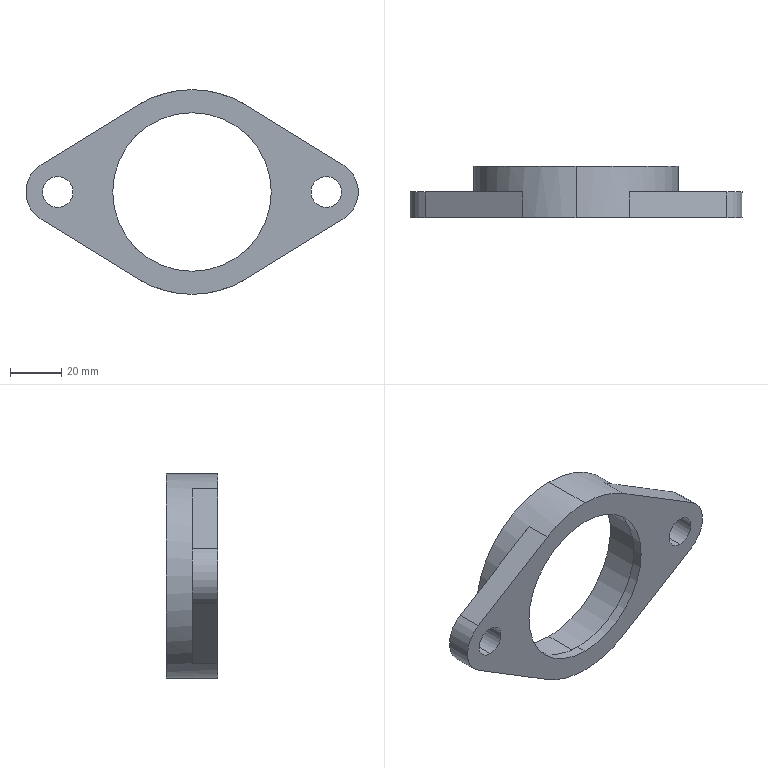Part | SolidWorks | features ICE 3, Extrusion 1 | 1 solid | 21 faces | box 130 x 20 x 80 mm | volume 45606 mm3 | cylinder 12 | plane 9 | commonest cylinder face diameters 12 x4 25 x2 62 x2 68 x2 80 x2
STEP:
#1=CARTESIAN_POINT('',(0.,0.,-31.));
#2=VERTEX_POINT('',#1);
#3=CARTESIAN_POINT('',(0.,0.,31.));
#4=VERTEX_POINT('',#3);
#5=CARTESIAN_POINT('',(0.,0.,0.));
#6=DIRECTION('',(0.,1.,0.));
#7=DIRECTION('',(0.,0.,1.));
#8=AXIS2_PLACEMENT_3D('',#5,#6,#7);
#9=CIRCLE('',#8,31.);
#10=EDGE_CURVE('',#2,#4,#9,.T.);
#11=ORIENTED_EDGE('',*,*,#10,.F.);
#12=CARTESIAN_POINT('',(0.,4.,-31.));
#13=VERTEX_POINT('',#12);
#14=CARTESIAN_POINT('',(0.,-12.,-31.));
#15=DIRECTION('',(0.,1.,0.));
#16=VECTOR('',#15,1000.);
#17=LINE('',#14,#16);
#18=EDGE_CURVE('',#2,#13,#17,.T.);
#19=ORIENTED_EDGE('',*,*,#18,.T.);
#20=CARTESIAN_POINT('',(0.,4.,31.));
#21=VERTEX_POINT('',#20);
#22=CARTESIAN_POINT('',(0.,4.,0.));
#23=DIRECTION('',(0.,1.,0.));
#24=DIRECTION('',(0.,0.,1.));
#25=AXIS2_PLACEMENT_3D('',#22,#23,#24);
#26=CIRCLE('',#25,31.);
#27=EDGE_CURVE('',#13,#21,#26,.T.);
#28=ORIENTED_EDGE('',*,*,#27,.T.);
#29=CARTESIAN_POINT('',(0.,-12.,31.));
#30=DIRECTION('',(0.,1.,0.));
#31=VECTOR('',#30,1000.);
#32=LINE('',#29,#31);
#33=EDGE_CURVE('',#4,#21,#32,.T.);
#34=ORIENTED_EDGE('',*,*,#33,.F.);
#35=EDGE_LOOP('',(#11,#19,#28,#34));
#36=FACE_OUTER_BOUND('',#35,.T.);
#37=CARTESIAN_POINT('',(0.,-12.,0.));
#38=DIRECTION('',(0.,1.,0.));
#39=DIRECTION('',(0.,0.,1.));
#40=AXIS2_PLACEMENT_3D('',#37,#38,#39);
#41=CYLINDRICAL_SURFACE('',#40,31.);
#42=ADVANCED_FACE('',(#36),#41,.F.);
#43=CARTESIAN_POINT('',(0.,4.,-34.));
#44=VERTEX_POINT('',#43);
#45=CARTESIAN_POINT('',(0.,4.,34.));
#46=VERTEX_POINT('',#45);
#47=CARTESIAN_POINT('',(0.,4.,0.));
#48=DIRECTION('',(0.,1.,0.));
#49=DIRECTION('',(0.,0.,1.));
#50=AXIS2_PLACEMENT_3D('',#47,#48,#49);
#51=CIRCLE('',#50,34.);
#52=EDGE_CURVE('',#44,#46,#51,.T.);
#53=ORIENTED_EDGE('',*,*,#52,.F.);
#54=CARTESIAN_POINT('',(0.,20.,-34.));
#55=VERTEX_POINT('',#54);
#56=CARTESIAN_POINT('',(0.,4.,-34.));
#57=DIRECTION('',(0.,1.,0.));
#58=VECTOR('',#57,1000.);
#59=LINE('',#56,#58);
#60=EDGE_CURVE('',#44,#55,#59,.T.);
#61=ORIENTED_EDGE('',*,*,#60,.T.);
#62=CARTESIAN_POINT('',(0.,20.,34.));
#63=VERTEX_POINT('',#62);
#64=CARTESIAN_POINT('',(0.,20.,0.));
#65=DIRECTION('',(0.,1.,0.));
#66=DIRECTION('',(0.,0.,1.));
#67=AXIS2_PLACEMENT_3D('',#64,#65,#66);
#68=CIRCLE('',#67,34.);
#69=EDGE_CURVE('',#55,#63,#68,.T.);
#70=ORIENTED_EDGE('',*,*,#69,.T.);
#71=CARTESIAN_POINT('',(0.,4.,34.));
#72=DIRECTION('',(0.,1.,0.));
#73=VECTOR('',#72,1000.);
#74=LINE('',#71,#73);
#75=EDGE_CURVE('',#46,#63,#74,.T.);
#76=ORIENTED_EDGE('',*,*,#75,.F.);
#77=EDGE_LOOP('',(#53,#61,#70,#76));
#78=FACE_OUTER_BOUND('',#77,.T.);
#79=CARTESIAN_POINT('',(0.,4.,0.));
#80=DIRECTION('',(0.,1.,0.));
#81=DIRECTION('',(0.,0.,1.));
#82=AXIS2_PLACEMENT_3D('',#79,#80,#81);
#83=CYLINDRICAL_SURFACE('',#82,34.);
#84=ADVANCED_FACE('',(#78),#83,.F.);
#85=CARTESIAN_POINT('',(-52.5,10.,-6.));
#86=VERTEX_POINT('',#85);
#87=CARTESIAN_POINT('',(-52.5,10.,6.));
#88=VERTEX_POINT('',#87);
#89=CARTESIAN_POINT('',(-52.5,10.,0.));
#90=DIRECTION('',(0.,1.,0.));
#91=DIRECTION('',(0.,0.,1.));
#92=AXIS2_PLACEMENT_3D('',#89,#90,#91);
#93=CIRCLE('',#92,6.);
#94=EDGE_CURVE('',#86,#88,#93,.T.);
#95=ORIENTED_EDGE('',*,*,#94,.T.);
#96=CARTESIAN_POINT('',(-52.5,0.,6.));
#97=VERTEX_POINT('',#96);
#98=CARTESIAN_POINT('',(-52.5,10.,6.));
#99=DIRECTION('',(0.,-1.,0.));
#100=VECTOR('',#99,1000.);
#101=LINE('',#98,#100);
#102=EDGE_CURVE('',#88,#97,#101,.T.);
#103=ORIENTED_EDGE('',*,*,#102,.T.);
#104=CARTESIAN_POINT('',(-52.5,0.,-6.));
#105=VERTEX_POINT('',#104);
#106=CARTESIAN_POINT('',(-52.5,0.,0.));
#107=DIRECTION('',(0.,1.,0.));
#108=DIRECTION('',(0.,0.,1.));
#109=AXIS2_PLACEMENT_3D('',#106,#107,#108);
#110=CIRCLE('',#109,6.);
#111=EDGE_CURVE('',#105,#97,#110,.T.);
#112=ORIENTED_EDGE('',*,*,#111,.F.);
#113=CARTESIAN_POINT('',(-52.5,10.,-6.));
#114=DIRECTION('',(0.,-1.,0.));
#115=VECTOR('',#114,1000.);
#116=LINE('',#113,#115);
#117=EDGE_CURVE('',#86,#105,#116,.T.);
#118=ORIENTED_EDGE('',*,*,#117,.F.);
#119=EDGE_LOOP('',(#95,#103,#112,#118));
#120=FACE_OUTER_BOUND('',#119,.T.);
#121=CARTESIAN_POINT('',(-52.5,10.,0.));
#122=DIRECTION('',(0.,-1.,0.));
#123=DIRECTION('',(0.,0.,-1.));
#124=AXIS2_PLACEMENT_3D('',#121,#122,#123);
#125=CYLINDRICAL_SURFACE('',#124,6.);
#126=ADVANCED_FACE('',(#120),#125,.F.);
#127=CARTESIAN_POINT('',(52.5,10.,-6.));
#128=VERTEX_POINT('',#127);
#129=CARTESIAN_POINT('',(52.5,10.,6.));
#130=VERTEX_POINT('',#129);
#131=CARTESIAN_POINT('',(52.5,10.,0.));
#132=DIRECTION('',(0.,1.,0.));
#133=DIRECTION('',(0.,0.,1.));
#134=AXIS2_PLACEMENT_3D('',#131,#132,#133);
#135=CIRCLE('',#134,6.);
#136=EDGE_CURVE('',#128,#130,#135,.T.);
#137=ORIENTED_EDGE('',*,*,#136,.T.);
#138=CARTESIAN_POINT('',(52.5,0.,6.));
#139=VERTEX_POINT('',#138);
#140=CARTESIAN_POINT('',(52.5,10.,6.));
#141=DIRECTION('',(0.,-1.,0.));
#142=VECTOR('',#141,1000.);
#143=LINE('',#140,#142);
#144=EDGE_CURVE('',#130,#139,#143,.T.);
#145=ORIENTED_EDGE('',*,*,#144,.T.);
#146=CARTESIAN_POINT('',(52.5,0.,-6.));
#147=VERTEX_POINT('',#146);
#148=CARTESIAN_POINT('',(52.5,0.,0.));
#149=DIRECTION('',(0.,1.,0.));
#150=DIRECTION('',(0.,0.,1.));
#151=AXIS2_PLACEMENT_3D('',#148,#149,#150);
#152=CIRCLE('',#151,6.);
#153=EDGE_CURVE('',#147,#139,#152,.T.);
#154=ORIENTED_EDGE('',*,*,#153,.F.);
#155=CARTESIAN_POINT('',(52.5,10.,-6.));
#156=DIRECTION('',(0.,-1.,0.));
#157=VECTOR('',#156,1000.);
#158=LINE('',#155,#157);
#159=EDGE_CURVE('',#128,#147,#158,.T.);
#160=ORIENTED_EDGE('',*,*,#159,.F.);
#161=EDGE_LOOP('',(#137,#145,#154,#160));
#162=FACE_OUTER_BOUND('',#161,.T.);
#163=CARTESIAN_POINT('',(52.5,10.,0.));
#164=DIRECTION('',(0.,-1.,0.));
#165=DIRECTION('',(0.,0.,-1.));
#166=AXIS2_PLACEMENT_3D('',#163,#164,#165);
#167=CYLINDRICAL_SURFACE('',#166,6.);
#168=ADVANCED_FACE('',(#162),#167,.F.);
#169=CARTESIAN_POINT('',(0.,20.,40.));
#170=VERTEX_POINT('',#169);
#171=CARTESIAN_POINT('',(0.,20.,-40.));
#172=VERTEX_POINT('',#171);
#173=CARTESIAN_POINT('',(0.,20.,0.));
#174=DIRECTION('',(0.,1.,0.));
#175=DIRECTION('',(0.,0.,1.));
#176=AXIS2_PLACEMENT_3D('',#173,#174,#175);
#177=CIRCLE('',#176,40.);
#178=EDGE_CURVE('',#170,#172,#177,.T.);
#179=ORIENTED_EDGE('',*,*,#178,.F.);
#180=CARTESIAN_POINT('',(0.,0.,40.));
#181=VERTEX_POINT('',#180);
#182=CARTESIAN_POINT('',(0.,10.,40.));
#183=DIRECTION('',(0.,-1.,0.));
#184=VECTOR('',#183,1000.);
#185=LINE('',#182,#184);
#186=EDGE_CURVE('',#170,#181,#185,.T.);
#187=ORIENTED_EDGE('',*,*,#186,.T.);
#188=CARTESIAN_POINT('',(20.952,0.,34.073));
#189=VERTEX_POINT('',#188);
#190=CARTESIAN_POINT('',(0.,0.,0.));
#191=DIRECTION('',(0.,1.,0.));
#192=DIRECTION('',(0.,0.,1.));
#193=AXIS2_PLACEMENT_3D('',#190,#191,#192);
#194=CIRCLE('',#193,40.);
#195=EDGE_CURVE('',#181,#189,#194,.T.);
#196=ORIENTED_EDGE('',*,*,#195,.T.);
#197=CARTESIAN_POINT('',(20.952,10.,34.073));
#198=VERTEX_POINT('',#197);
#199=CARTESIAN_POINT('',(20.952,10.,34.073));
#200=DIRECTION('',(0.,-1.,0.));
#201=VECTOR('',#200,1000.);
#202=LINE('',#199,#201);
#203=EDGE_CURVE('',#198,#189,#202,.T.);
#204=ORIENTED_EDGE('',*,*,#203,.F.);
#205=CARTESIAN_POINT('',(20.952,10.,-34.073));
#206=VERTEX_POINT('',#205);
#207=CARTESIAN_POINT('',(0.,10.,0.));
#208=DIRECTION('',(0.,1.,0.));
#209=DIRECTION('',(0.,0.,1.));
#210=AXIS2_PLACEMENT_3D('',#207,#208,#209);
#211=CIRCLE('',#210,40.);
#212=EDGE_CURVE('',#198,#206,#211,.T.);
#213=ORIENTED_EDGE('',*,*,#212,.T.);
#214=CARTESIAN_POINT('',(20.952,0.,-34.073));
#215=VERTEX_POINT('',#214);
#216=CARTESIAN_POINT('',(20.952,10.,-34.073));
#217=DIRECTION('',(0.,-1.,0.));
#218=VECTOR('',#217,1000.);
#219=LINE('',#216,#218);
#220=EDGE_CURVE('',#206,#215,#219,.T.);
#221=ORIENTED_EDGE('',*,*,#220,.T.);
#222=CARTESIAN_POINT('',(0.,0.,-40.));
#223=VERTEX_POINT('',#222);
#224=CARTESIAN_POINT('',(0.,0.,0.));
#225=DIRECTION('',(0.,1.,0.));
#226=DIRECTION('',(0.,0.,1.));
#227=AXIS2_PLACEMENT_3D('',#224,#225,#226);
#228=CIRCLE('',#227,40.);
#229=EDGE_CURVE('',#215,#223,#228,.T.);
#230=ORIENTED_EDGE('',*,*,#229,.T.);
#231=CARTESIAN_POINT('',(0.,10.,-40.));
#232=DIRECTION('',(0.,-1.,0.));
#233=VECTOR('',#232,1000.);
#234=LINE('',#231,#233);
#235=EDGE_CURVE('',#172,#223,#234,.T.);
#236=ORIENTED_EDGE('',*,*,#235,.F.);
#237=EDGE_LOOP('',(#179,#187,#196,#204,#213,#221,#230,#236));
#238=FACE_OUTER_BOUND('',#237,.T.);
#239=CARTESIAN_POINT('',(0.,10.,0.));
#240=DIRECTION('',(0.,-1.,0.));
#241=DIRECTION('',(0.,0.,-1.));
#242=AXIS2_PLACEMENT_3D('',#239,#240,#241);
#243=CYLINDRICAL_SURFACE('',#242,40.);
#244=ADVANCED_FACE('',(#238),#243,.T.);
#245=ORIENTED_EDGE('',*,*,#212,.F.);
#246=CARTESIAN_POINT('',(59.048,10.,10.648));
#247=VERTEX_POINT('',#246);
#248=CARTESIAN_POINT('',(59.048,10.,10.648));
#249=DIRECTION('',(0.8518,0.,-0.5238));
#250=VECTOR('',#249,1000.);
#251=LINE('',#248,#250);
#252=EDGE_CURVE('',#198,#247,#251,.T.);
#253=ORIENTED_EDGE('',*,*,#252,.T.);
#254=CARTESIAN_POINT('',(59.048,10.,-10.648));
#255=VERTEX_POINT('',#254);
#256=CARTESIAN_POINT('',(52.5,10.,0.));
#257=DIRECTION('',(0.,1.,0.));
#258=DIRECTION('',(0.,0.,1.));
#259=AXIS2_PLACEMENT_3D('',#256,#257,#258);
#260=CIRCLE('',#259,12.5);
#261=EDGE_CURVE('',#247,#255,#260,.T.);
#262=ORIENTED_EDGE('',*,*,#261,.T.);
#263=CARTESIAN_POINT('',(20.952,10.,-34.073));
#264=DIRECTION('',(-0.8518,0.,-0.5238));
#265=VECTOR('',#264,1000.);
#266=LINE('',#263,#265);
#267=EDGE_CURVE('',#255,#206,#266,.T.);
#268=ORIENTED_EDGE('',*,*,#267,.T.);
#269=EDGE_LOOP('',(#245,#253,#262,#268));
#270=FACE_OUTER_BOUND('',#269,.T.);
#271=ORIENTED_EDGE('',*,*,#136,.F.);
#272=CARTESIAN_POINT('',(52.5,10.,0.));
#273=DIRECTION('',(0.,1.,0.));
#274=DIRECTION('',(0.,0.,1.));
#275=AXIS2_PLACEMENT_3D('',#272,#273,#274);
#276=CIRCLE('',#275,6.);
#277=EDGE_CURVE('',#130,#128,#276,.T.);
#278=ORIENTED_EDGE('',*,*,#277,.F.);
#279=EDGE_LOOP('',(#271,#278));
#280=FACE_BOUND('',#279,.T.);
#281=CARTESIAN_POINT('',(-52.5,10.,0.));
#282=DIRECTION('',(0.,1.,0.));
#283=DIRECTION('',(0.,0.,1.));
#284=AXIS2_PLACEMENT_3D('',#281,#282,#283);
#285=PLANE('',#284);
#286=ADVANCED_FACE('',(#270,#280),#285,.T.);
#287=CARTESIAN_POINT('',(-20.952,10.,-34.073));
#288=VERTEX_POINT('',#287);
#289=CARTESIAN_POINT('',(-20.952,10.,34.073));
#290=VERTEX_POINT('',#289);
#291=CARTESIAN_POINT('',(0.,10.,0.));
#292=DIRECTION('',(0.,1.,0.));
#293=DIRECTION('',(0.,0.,1.));
#294=AXIS2_PLACEMENT_3D('',#291,#292,#293);
#295=CIRCLE('',#294,40.);
#296=EDGE_CURVE('',#288,#290,#295,.T.);
#297=ORIENTED_EDGE('',*,*,#296,.F.);
#298=CARTESIAN_POINT('',(-59.048,10.,-10.648));
#299=VERTEX_POINT('',#298);
#300=CARTESIAN_POINT('',(-59.048,10.,-10.648));
#301=DIRECTION('',(-0.8518,0.,0.5238));
#302=VECTOR('',#301,1000.);
#303=LINE('',#300,#302);
#304=EDGE_CURVE('',#288,#299,#303,.T.);
#305=ORIENTED_EDGE('',*,*,#304,.T.);
#306=CARTESIAN_POINT('',(-59.048,10.,10.648));
#307=VERTEX_POINT('',#306);
#308=CARTESIAN_POINT('',(-52.5,10.,0.));
#309=DIRECTION('',(0.,1.,0.));
#310=DIRECTION('',(0.,0.,1.));
#311=AXIS2_PLACEMENT_3D('',#308,#309,#310);
#312=CIRCLE('',#311,12.5);
#313=EDGE_CURVE('',#299,#307,#312,.T.);
#314=ORIENTED_EDGE('',*,*,#313,.T.);
#315=CARTESIAN_POINT('',(-20.952,10.,34.073));
#316=DIRECTION('',(0.8518,0.,0.5238));
#317=VECTOR('',#316,1000.);
#318=LINE('',#315,#317);
#319=EDGE_CURVE('',#307,#290,#318,.T.);
#320=ORIENTED_EDGE('',*,*,#319,.T.);
#321=EDGE_LOOP('',(#297,#305,#314,#320));
#322=FACE_OUTER_BOUND('',#321,.T.);
#323=ORIENTED_EDGE('',*,*,#94,.F.);
#324=CARTESIAN_POINT('',(-52.5,10.,0.));
#325=DIRECTION('',(0.,1.,0.));
#326=DIRECTION('',(0.,0.,1.));
#327=AXIS2_PLACEMENT_3D('',#324,#325,#326);
#328=CIRCLE('',#327,6.);
#329=EDGE_CURVE('',#88,#86,#328,.T.);
#330=ORIENTED_EDGE('',*,*,#329,.F.);
#331=EDGE_LOOP('',(#323,#330));
#332=FACE_BOUND('',#331,.T.);
#333=CARTESIAN_POINT('',(-52.5,10.,0.));
#334=DIRECTION('',(0.,1.,0.));
#335=DIRECTION('',(0.,0.,1.));
#336=AXIS2_PLACEMENT_3D('',#333,#334,#335);
#337=PLANE('',#336);
#338=ADVANCED_FACE('',(#322,#332),#337,.T.);
#339=CARTESIAN_POINT('',(0.,0.,0.));
#340=DIRECTION('',(0.,1.,0.));
#341=DIRECTION('',(0.,0.,1.));
#342=AXIS2_PLACEMENT_3D('',#339,#340,#341);
#343=CIRCLE('',#342,31.);
#344=EDGE_CURVE('',#4,#2,#343,.T.);
#345=ORIENTED_EDGE('',*,*,#344,.T.);
#346=ORIENTED_EDGE('',*,*,#10,.T.);
#347=EDGE_LOOP('',(#345,#346));
#348=FACE_BOUND('',#347,.T.);
#349=ORIENTED_EDGE('',*,*,#153,.T.);
#350=CARTESIAN_POINT('',(52.5,0.,0.));
#351=DIRECTION('',(0.,1.,0.));
#352=DIRECTION('',(0.,0.,1.));
#353=AXIS2_PLACEMENT_3D('',#350,#351,#352);
#354=CIRCLE('',#353,6.);
#355=EDGE_CURVE('',#139,#147,#354,.T.);
#356=ORIENTED_EDGE('',*,*,#355,.T.);
#357=EDGE_LOOP('',(#349,#356));
#358=FACE_BOUND('',#357,.T.);
#359=CARTESIAN_POINT('',(-59.048,0.,-10.648));
#360=VERTEX_POINT('',#359);
#361=CARTESIAN_POINT('',(-59.048,0.,10.648));
#362=VERTEX_POINT('',#361);
#363=CARTESIAN_POINT('',(-52.5,0.,0.));
#364=DIRECTION('',(0.,1.,0.));
#365=DIRECTION('',(0.,0.,1.));
#366=AXIS2_PLACEMENT_3D('',#363,#364,#365);
#367=CIRCLE('',#366,12.5);
#368=EDGE_CURVE('',#360,#362,#367,.T.);
#369=ORIENTED_EDGE('',*,*,#368,.F.);
#370=CARTESIAN_POINT('',(-20.952,0.,-34.073));
#371=VERTEX_POINT('',#370);
#372=CARTESIAN_POINT('',(-59.048,0.,-10.648));
#373=DIRECTION('',(-0.8518,0.,0.5238));
#374=VECTOR('',#373,1000.);
#375=LINE('',#372,#374);
#376=EDGE_CURVE('',#371,#360,#375,.T.);
#377=ORIENTED_EDGE('',*,*,#376,.F.);
#378=CARTESIAN_POINT('',(0.,0.,0.));
#379=DIRECTION('',(0.,1.,0.));
#380=DIRECTION('',(0.,0.,1.));
#381=AXIS2_PLACEMENT_3D('',#378,#379,#380);
#382=CIRCLE('',#381,40.);
#383=EDGE_CURVE('',#223,#371,#382,.T.);
#384=ORIENTED_EDGE('',*,*,#383,.F.);
#385=ORIENTED_EDGE('',*,*,#229,.F.);
#386=CARTESIAN_POINT('',(59.048,0.,-10.648));
#387=VERTEX_POINT('',#386);
#388=CARTESIAN_POINT('',(20.952,0.,-34.073));
#389=DIRECTION('',(-0.8518,0.,-0.5238));
#390=VECTOR('',#389,1000.);
#391=LINE('',#388,#390);
#392=EDGE_CURVE('',#387,#215,#391,.T.);
#393=ORIENTED_EDGE('',*,*,#392,.F.);
#394=CARTESIAN_POINT('',(59.048,0.,10.648));
#395=VERTEX_POINT('',#394);
#396=CARTESIAN_POINT('',(52.5,0.,0.));
#397=DIRECTION('',(0.,1.,0.));
#398=DIRECTION('',(0.,0.,1.));
#399=AXIS2_PLACEMENT_3D('',#396,#397,#398);
#400=CIRCLE('',#399,12.5);
#401=EDGE_CURVE('',#395,#387,#400,.T.);
#402=ORIENTED_EDGE('',*,*,#401,.F.);
#403=CARTESIAN_POINT('',(59.048,0.,10.648));
#404=DIRECTION('',(0.8518,0.,-0.5238));
#405=VECTOR('',#404,1000.);
#406=LINE('',#403,#405);
#407=EDGE_CURVE('',#189,#395,#406,.T.);
#408=ORIENTED_EDGE('',*,*,#407,.F.);
#409=ORIENTED_EDGE('',*,*,#195,.F.);
#410=CARTESIAN_POINT('',(-20.952,0.,34.073));
#411=VERTEX_POINT('',#410);
#412=CARTESIAN_POINT('',(0.,0.,0.));
#413=DIRECTION('',(0.,1.,0.));
#414=DIRECTION('',(0.,0.,1.));
#415=AXIS2_PLACEMENT_3D('',#412,#413,#414);
#416=CIRCLE('',#415,40.);
#417=EDGE_CURVE('',#411,#181,#416,.T.);
#418=ORIENTED_EDGE('',*,*,#417,.F.);
#419=CARTESIAN_POINT('',(-20.952,0.,34.073));
#420=DIRECTION('',(0.8518,0.,0.5238));
#421=VECTOR('',#420,1000.);
#422=LINE('',#419,#421);
#423=EDGE_CURVE('',#362,#411,#422,.T.);
#424=ORIENTED_EDGE('',*,*,#423,.F.);
#425=EDGE_LOOP('',(#369,#377,#384,#385,#393,#402,#408,#409,#418,#424));
#426=FACE_OUTER_BOUND('',#425,.T.);
#427=ORIENTED_EDGE('',*,*,#111,.T.);
#428=CARTESIAN_POINT('',(-52.5,0.,0.));
#429=DIRECTION('',(0.,1.,0.));
#430=DIRECTION('',(0.,0.,1.));
#431=AXIS2_PLACEMENT_3D('',#428,#429,#430);
#432=CIRCLE('',#431,6.);
#433=EDGE_CURVE('',#97,#105,#432,.T.);
#434=ORIENTED_EDGE('',*,*,#433,.T.);
#435=EDGE_LOOP('',(#427,#434));
#436=FACE_BOUND('',#435,.T.);
#437=CARTESIAN_POINT('',(-52.5,0.,0.));
#438=DIRECTION('',(0.,1.,0.));
#439=DIRECTION('',(0.,0.,1.));
#440=AXIS2_PLACEMENT_3D('',#437,#438,#439);
#441=PLANE('',#440);
#442=ADVANCED_FACE('',(#348,#358,#426,#436),#441,.F.);
#443=ORIENTED_EDGE('',*,*,#368,.T.);
#444=CARTESIAN_POINT('',(-59.048,10.,10.648));
#445=DIRECTION('',(0.,-1.,0.));
#446=VECTOR('',#445,1000.);
#447=LINE('',#444,#446);
#448=EDGE_CURVE('',#307,#362,#447,.T.);
#449=ORIENTED_EDGE('',*,*,#448,.F.);
#450=ORIENTED_EDGE('',*,*,#313,.F.);
#451=CARTESIAN_POINT('',(-59.048,10.,-10.648));
#452=DIRECTION('',(0.,-1.,0.));
#453=VECTOR('',#452,1000.);
#454=LINE('',#451,#453);
#455=EDGE_CURVE('',#299,#360,#454,.T.);
#456=ORIENTED_EDGE('',*,*,#455,.T.);
#457=EDGE_LOOP('',(#443,#449,#450,#456));
#458=FACE_OUTER_BOUND('',#457,.T.);
#459=CARTESIAN_POINT('',(-52.5,10.,0.));
#460=DIRECTION('',(0.,-1.,0.));
#461=DIRECTION('',(0.,0.,-1.));
#462=AXIS2_PLACEMENT_3D('',#459,#460,#461);
#463=CYLINDRICAL_SURFACE('',#462,12.5);
#464=ADVANCED_FACE('',(#458),#463,.T.);
#465=ORIENTED_EDGE('',*,*,#423,.T.);
#466=CARTESIAN_POINT('',(-20.952,10.,34.073));
#467=DIRECTION('',(0.,-1.,0.));
#468=VECTOR('',#467,1000.);
#469=LINE('',#466,#468);
#470=EDGE_CURVE('',#290,#411,#469,.T.);
#471=ORIENTED_EDGE('',*,*,#470,.F.);
#472=ORIENTED_EDGE('',*,*,#319,.F.);
#473=ORIENTED_EDGE('',*,*,#448,.T.);
#474=EDGE_LOOP('',(#465,#471,#472,#473));
#475=FACE_OUTER_BOUND('',#474,.T.);
#476=CARTESIAN_POINT('',(-20.952,10.,34.073));
#477=DIRECTION('',(0.5238,0.,-0.8518));
#478=DIRECTION('',(-0.8518,0.,-0.5238));
#479=AXIS2_PLACEMENT_3D('',#476,#477,#478);
#480=PLANE('',#479);
#481=ADVANCED_FACE('',(#475),#480,.F.);
#482=ORIENTED_EDGE('',*,*,#407,.T.);
#483=CARTESIAN_POINT('',(59.048,10.,10.648));
#484=DIRECTION('',(0.,-1.,0.));
#485=VECTOR('',#484,1000.);
#486=LINE('',#483,#485);
#487=EDGE_CURVE('',#247,#395,#486,.T.);
#488=ORIENTED_EDGE('',*,*,#487,.F.);
#489=ORIENTED_EDGE('',*,*,#252,.F.);
#490=ORIENTED_EDGE('',*,*,#203,.T.);
#491=EDGE_LOOP('',(#482,#488,#489,#490));
#492=FACE_OUTER_BOUND('',#491,.T.);
#493=CARTESIAN_POINT('',(59.048,10.,10.648));
#494=DIRECTION('',(-0.5238,0.,-0.8518));
#495=DIRECTION('',(-0.8518,0.,0.5238));
#496=AXIS2_PLACEMENT_3D('',#493,#494,#495);
#497=PLANE('',#496);
#498=ADVANCED_FACE('',(#492),#497,.F.);
#499=ORIENTED_EDGE('',*,*,#401,.T.);
#500=CARTESIAN_POINT('',(59.048,10.,-10.648));
#501=DIRECTION('',(0.,-1.,0.));
#502=VECTOR('',#501,1000.);
#503=LINE('',#500,#502);
#504=EDGE_CURVE('',#255,#387,#503,.T.);
#505=ORIENTED_EDGE('',*,*,#504,.F.);
#506=ORIENTED_EDGE('',*,*,#261,.F.);
#507=ORIENTED_EDGE('',*,*,#487,.T.);
#508=EDGE_LOOP('',(#499,#505,#506,#507));
#509=FACE_OUTER_BOUND('',#508,.T.);
#510=CARTESIAN_POINT('',(52.5,10.,0.));
#511=DIRECTION('',(0.,-1.,0.));
#512=DIRECTION('',(0.,0.,-1.));
#513=AXIS2_PLACEMENT_3D('',#510,#511,#512);
#514=CYLINDRICAL_SURFACE('',#513,12.5);
#515=ADVANCED_FACE('',(#509),#514,.T.);
#516=ORIENTED_EDGE('',*,*,#392,.T.);
#517=ORIENTED_EDGE('',*,*,#220,.F.);
#518=ORIENTED_EDGE('',*,*,#267,.F.);
#519=ORIENTED_EDGE('',*,*,#504,.T.);
#520=EDGE_LOOP('',(#516,#517,#518,#519));
#521=FACE_OUTER_BOUND('',#520,.T.);
#522=CARTESIAN_POINT('',(20.952,10.,-34.073));
#523=DIRECTION('',(-0.5238,0.,0.8518));
#524=DIRECTION('',(0.8518,0.,0.5238));
#525=AXIS2_PLACEMENT_3D('',#522,#523,#524);
#526=PLANE('',#525);
#527=ADVANCED_FACE('',(#521),#526,.F.);
#528=ORIENTED_EDGE('',*,*,#186,.F.);
#529=CARTESIAN_POINT('',(0.,20.,0.));
#530=DIRECTION('',(0.,1.,0.));
#531=DIRECTION('',(0.,0.,1.));
#532=AXIS2_PLACEMENT_3D('',#529,#530,#531);
#533=CIRCLE('',#532,40.);
#534=EDGE_CURVE('',#172,#170,#533,.T.);
#535=ORIENTED_EDGE('',*,*,#534,.F.);
#536=ORIENTED_EDGE('',*,*,#235,.T.);
#537=ORIENTED_EDGE('',*,*,#383,.T.);
#538=CARTESIAN_POINT('',(-20.952,10.,-34.073));
#539=DIRECTION('',(0.,-1.,0.));
#540=VECTOR('',#539,1000.);
#541=LINE('',#538,#540);
#542=EDGE_CURVE('',#288,#371,#541,.T.);
#543=ORIENTED_EDGE('',*,*,#542,.F.);
#544=ORIENTED_EDGE('',*,*,#296,.T.);
#545=ORIENTED_EDGE('',*,*,#470,.T.);
#546=ORIENTED_EDGE('',*,*,#417,.T.);
#547=EDGE_LOOP('',(#528,#535,#536,#537,#543,#544,#545,#546));
#548=FACE_OUTER_BOUND('',#547,.T.);
#549=CARTESIAN_POINT('',(0.,10.,0.));
#550=DIRECTION('',(0.,-1.,0.));
#551=DIRECTION('',(0.,0.,-1.));
#552=AXIS2_PLACEMENT_3D('',#549,#550,#551);
#553=CYLINDRICAL_SURFACE('',#552,40.);
#554=ADVANCED_FACE('',(#548),#553,.T.);
#555=ORIENTED_EDGE('',*,*,#376,.T.);
#556=ORIENTED_EDGE('',*,*,#455,.F.);
#557=ORIENTED_EDGE('',*,*,#304,.F.);
#558=ORIENTED_EDGE('',*,*,#542,.T.);
#559=EDGE_LOOP('',(#555,#556,#557,#558));
#560=FACE_OUTER_BOUND('',#559,.T.);
#561=CARTESIAN_POINT('',(-59.048,10.,-10.648));
#562=DIRECTION('',(0.5238,0.,0.8518));
#563=DIRECTION('',(0.8518,0.,-0.5238));
#564=AXIS2_PLACEMENT_3D('',#561,#562,#563);
#565=PLANE('',#564);
#566=ADVANCED_FACE('',(#560),#565,.F.);
#567=ORIENTED_EDGE('',*,*,#144,.F.);
#568=ORIENTED_EDGE('',*,*,#277,.T.);
#569=ORIENTED_EDGE('',*,*,#159,.T.);
#570=ORIENTED_EDGE('',*,*,#355,.F.);
#571=EDGE_LOOP('',(#567,#568,#569,#570));
#572=FACE_OUTER_BOUND('',#571,.T.);
#573=CARTESIAN_POINT('',(52.5,10.,0.));
#574=DIRECTION('',(0.,-1.,0.));
#575=DIRECTION('',(0.,0.,-1.));
#576=AXIS2_PLACEMENT_3D('',#573,#574,#575);
#577=CYLINDRICAL_SURFACE('',#576,6.);
#578=ADVANCED_FACE('',(#572),#577,.F.);
#579=ORIENTED_EDGE('',*,*,#102,.F.);
#580=ORIENTED_EDGE('',*,*,#329,.T.);
#581=ORIENTED_EDGE('',*,*,#117,.T.);
#582=ORIENTED_EDGE('',*,*,#433,.F.);
#583=EDGE_LOOP('',(#579,#580,#581,#582));
#584=FACE_OUTER_BOUND('',#583,.T.);
#585=CARTESIAN_POINT('',(-52.5,10.,0.));
#586=DIRECTION('',(0.,-1.,0.));
#587=DIRECTION('',(0.,0.,-1.));
#588=AXIS2_PLACEMENT_3D('',#585,#586,#587);
#589=CYLINDRICAL_SURFACE('',#588,6.);
#590=ADVANCED_FACE('',(#584),#589,.F.);
#591=CARTESIAN_POINT('',(0.,20.,0.));
#592=DIRECTION('',(0.,1.,0.));
#593=DIRECTION('',(0.,0.,1.));
#594=AXIS2_PLACEMENT_3D('',#591,#592,#593);
#595=CIRCLE('',#594,34.);
#596=EDGE_CURVE('',#63,#55,#595,.T.);
#597=ORIENTED_EDGE('',*,*,#596,.F.);
#598=ORIENTED_EDGE('',*,*,#69,.F.);
#599=EDGE_LOOP('',(#597,#598));
#600=FACE_BOUND('',#599,.T.);
#601=ORIENTED_EDGE('',*,*,#534,.T.);
#602=ORIENTED_EDGE('',*,*,#178,.T.);
#603=EDGE_LOOP('',(#601,#602));
#604=FACE_OUTER_BOUND('',#603,.T.);
#605=CARTESIAN_POINT('',(0.,20.,0.));
#606=DIRECTION('',(0.,1.,0.));
#607=DIRECTION('',(0.,0.,1.));
#608=AXIS2_PLACEMENT_3D('',#605,#606,#607);
#609=PLANE('',#608);
#610=ADVANCED_FACE('',(#600,#604),#609,.T.);
#611=ORIENTED_EDGE('',*,*,#60,.F.);
#612=CARTESIAN_POINT('',(0.,4.,0.));
#613=DIRECTION('',(0.,1.,0.));
#614=DIRECTION('',(0.,0.,1.));
#615=AXIS2_PLACEMENT_3D('',#612,#613,#614);
#616=CIRCLE('',#615,34.);
#617=EDGE_CURVE('',#46,#44,#616,.T.);
#618=ORIENTED_EDGE('',*,*,#617,.F.);
#619=ORIENTED_EDGE('',*,*,#75,.T.);
#620=ORIENTED_EDGE('',*,*,#596,.T.);
#621=EDGE_LOOP('',(#611,#618,#619,#620));
#622=FACE_OUTER_BOUND('',#621,.T.);
#623=CARTESIAN_POINT('',(0.,4.,0.));
#624=DIRECTION('',(0.,1.,0.));
#625=DIRECTION('',(0.,0.,1.));
#626=AXIS2_PLACEMENT_3D('',#623,#624,#625);
#627=CYLINDRICAL_SURFACE('',#626,34.);
#628=ADVANCED_FACE('',(#622),#627,.F.);
#629=CARTESIAN_POINT('',(0.,4.,0.));
#630=DIRECTION('',(0.,1.,0.));
#631=DIRECTION('',(0.,0.,1.));
#632=AXIS2_PLACEMENT_3D('',#629,#630,#631);
#633=CIRCLE('',#632,31.);
#634=EDGE_CURVE('',#21,#13,#633,.T.);
#635=ORIENTED_EDGE('',*,*,#634,.F.);
#636=ORIENTED_EDGE('',*,*,#27,.F.);
#637=EDGE_LOOP('',(#635,#636));
#638=FACE_BOUND('',#637,.T.);
#639=ORIENTED_EDGE('',*,*,#617,.T.);
#640=ORIENTED_EDGE('',*,*,#52,.T.);
#641=EDGE_LOOP('',(#639,#640));
#642=FACE_OUTER_BOUND('',#641,.T.);
#643=CARTESIAN_POINT('',(0.,4.,0.));
#644=DIRECTION('',(0.,1.,0.));
#645=DIRECTION('',(0.,0.,1.));
#646=AXIS2_PLACEMENT_3D('',#643,#644,#645);
#647=PLANE('',#646);
#648=ADVANCED_FACE('',(#638,#642),#647,.T.);
#649=ORIENTED_EDGE('',*,*,#18,.F.);
#650=ORIENTED_EDGE('',*,*,#344,.F.);
#651=ORIENTED_EDGE('',*,*,#33,.T.);
#652=ORIENTED_EDGE('',*,*,#634,.T.);
#653=EDGE_LOOP('',(#649,#650,#651,#652));
#654=FACE_OUTER_BOUND('',#653,.T.);
#655=CARTESIAN_POINT('',(0.,-12.,0.));
#656=DIRECTION('',(0.,1.,0.));
#657=DIRECTION('',(0.,0.,1.));
#658=AXIS2_PLACEMENT_3D('',#655,#656,#657);
#659=CYLINDRICAL_SURFACE('',#658,31.);
#660=ADVANCED_FACE('',(#654),#659,.F.);
#661=CLOSED_SHELL('',(#42,#84,#126,#168,#244,#286,#338,#442,#464,#481,#498,#515,#527,#554,#566,#578,#590,#610,#628,#648,#660));
#662=MANIFOLD_SOLID_BREP('',#661);
#663=CARTESIAN_POINT('',(0.,0.,0.));
#664=DIRECTION('',(0.,0.,1.));
#665=DIRECTION('',(1.,0.,0.));
#666=AXIS2_PLACEMENT_3D('',#663,#664,#665);
#667=(LENGTH_UNIT()NAMED_UNIT(*)SI_UNIT(.MILLI.,.METRE.));
#668=UNCERTAINTY_MEASURE_WITH_UNIT(LENGTH_MEASURE(0.00001),#667,'','');
#669=(NAMED_UNIT(*)PLANE_ANGLE_UNIT()SI_UNIT($,.RADIAN.));
#670=(NAMED_UNIT(*)SI_UNIT($,.STERADIAN.)SOLID_ANGLE_UNIT());
#671=(GEOMETRIC_REPRESENTATION_CONTEXT(3)GLOBAL_UNCERTAINTY_ASSIGNED_CONTEXT((#668))GLOBAL_UNIT_ASSIGNED_CONTEXT((#667,#669,#670))REPRESENTATION_CONTEXT('',''));
#672=ADVANCED_BREP_SHAPE_REPRESENTATION('',(#662,#666),#671);